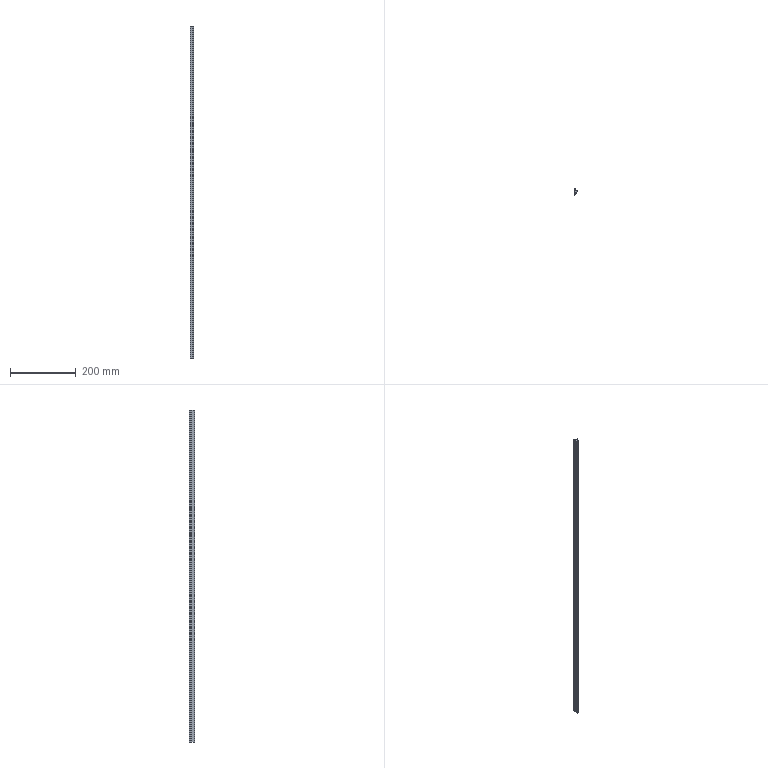Part | SolidWorks | features BaseBody 1, MoveFace 1 | 1 solid | 20 faces | box 10.8 x 17.5 x 1010 mm | volume 79589 mm3 | cylinder 11 | plane 9 | commonest cylinder face diameters 1.6 x2 14 x2 0.4 x1 0.6 x1 0.8 x1 2.6 x1
STEP:
#1=CARTESIAN_POINT('',(-3.236,-11.055,910.));
#2=VERTEX_POINT('',#1);
#3=CARTESIAN_POINT('',(-4.3,-10.3,910.));
#4=VERTEX_POINT('',#3);
#5=CARTESIAN_POINT('',(-3.5,-10.3,910.));
#6=DIRECTION('',(0.,0.,-1.));
#7=DIRECTION('',(1.,0.,0.));
#8=AXIS2_PLACEMENT_3D('',#5,#6,#7);
#9=CIRCLE('',#8,0.8);
#10=EDGE_CURVE('',#2,#4,#9,.T.);
#11=ORIENTED_EDGE('',*,*,#10,.T.);
#12=CARTESIAN_POINT('',(-4.3,-10.3,-100.));
#13=VERTEX_POINT('',#12);
#14=CARTESIAN_POINT('',(-4.3,-10.3,-100.));
#15=DIRECTION('',(0.,0.,-1.));
#16=VECTOR('',#15,1000.);
#17=LINE('',#14,#16);
#18=EDGE_CURVE('',#4,#13,#17,.T.);
#19=ORIENTED_EDGE('',*,*,#18,.T.);
#20=CARTESIAN_POINT('',(-3.236,-11.055,-100.));
#21=VERTEX_POINT('',#20);
#22=CARTESIAN_POINT('',(-3.5,-10.3,-100.));
#23=DIRECTION('',(0.,0.,1.));
#24=DIRECTION('',(-1.,0.,0.));
#25=AXIS2_PLACEMENT_3D('',#22,#23,#24);
#26=CIRCLE('',#25,0.8);
#27=EDGE_CURVE('',#13,#21,#26,.T.);
#28=ORIENTED_EDGE('',*,*,#27,.T.);
#29=CARTESIAN_POINT('',(-3.236,-11.055,-100.));
#30=DIRECTION('',(0.,0.,-1.));
#31=VECTOR('',#30,1000.);
#32=LINE('',#29,#31);
#33=EDGE_CURVE('',#2,#21,#32,.T.);
#34=ORIENTED_EDGE('',*,*,#33,.F.);
#35=EDGE_LOOP('',(#11,#19,#28,#34));
#36=FACE_OUTER_BOUND('',#35,.T.);
#37=CARTESIAN_POINT('',(-3.5,-10.3,-100.));
#38=DIRECTION('',(0.,0.,-1.));
#39=DIRECTION('',(-1.,0.,0.));
#40=AXIS2_PLACEMENT_3D('',#37,#38,#39);
#41=CYLINDRICAL_SURFACE('',#40,0.8);
#42=ADVANCED_FACE('',(#36),#41,.T.);
#43=CARTESIAN_POINT('',(1.184,-6.397,-100.));
#44=VERTEX_POINT('',#43);
#45=CARTESIAN_POINT('',(-5.702,-4.29,-100.));
#46=DIRECTION('',(0.,0.,1.));
#47=DIRECTION('',(-1.,0.,0.));
#48=AXIS2_PLACEMENT_3D('',#45,#46,#47);
#49=CIRCLE('',#48,7.201);
#50=EDGE_CURVE('',#21,#44,#49,.T.);
#51=ORIENTED_EDGE('',*,*,#50,.T.);
#52=CARTESIAN_POINT('',(1.184,-6.397,910.));
#53=VERTEX_POINT('',#52);
#54=CARTESIAN_POINT('',(1.184,-6.397,-100.));
#55=DIRECTION('',(0.,0.,1.));
#56=VECTOR('',#55,1000.);
#57=LINE('',#54,#56);
#58=EDGE_CURVE('',#44,#53,#57,.T.);
#59=ORIENTED_EDGE('',*,*,#58,.T.);
#60=CARTESIAN_POINT('',(-5.702,-4.29,910.));
#61=DIRECTION('',(0.,0.,-1.));
#62=DIRECTION('',(1.,0.,0.));
#63=AXIS2_PLACEMENT_3D('',#60,#61,#62);
#64=CIRCLE('',#63,7.201);
#65=EDGE_CURVE('',#53,#2,#64,.T.);
#66=ORIENTED_EDGE('',*,*,#65,.T.);
#67=ORIENTED_EDGE('',*,*,#33,.T.);
#68=EDGE_LOOP('',(#51,#59,#66,#67));
#69=FACE_OUTER_BOUND('',#68,.T.);
#70=CARTESIAN_POINT('',(-5.702,-4.29,-100.));
#71=DIRECTION('',(0.,0.,-1.));
#72=DIRECTION('',(-1.,0.,0.));
#73=AXIS2_PLACEMENT_3D('',#70,#71,#72);
#74=CYLINDRICAL_SURFACE('',#73,7.201);
#75=ADVANCED_FACE('',(#69),#74,.T.);
#76=CARTESIAN_POINT('',(0.9,-6.,-100.));
#77=VERTEX_POINT('',#76);
#78=CARTESIAN_POINT('',(0.9,-6.3,-100.));
#79=DIRECTION('',(0.,0.,1.));
#80=DIRECTION('',(-1.,0.,0.));
#81=AXIS2_PLACEMENT_3D('',#78,#79,#80);
#82=CIRCLE('',#81,0.3);
#83=EDGE_CURVE('',#44,#77,#82,.T.);
#84=ORIENTED_EDGE('',*,*,#83,.T.);
#85=CARTESIAN_POINT('',(0.9,-6.,910.));
#86=VERTEX_POINT('',#85);
#87=CARTESIAN_POINT('',(0.9,-6.,-100.));
#88=DIRECTION('',(0.,0.,1.));
#89=VECTOR('',#88,1000.);
#90=LINE('',#87,#89);
#91=EDGE_CURVE('',#77,#86,#90,.T.);
#92=ORIENTED_EDGE('',*,*,#91,.T.);
#93=CARTESIAN_POINT('',(0.9,-6.3,910.));
#94=DIRECTION('',(0.,0.,-1.));
#95=DIRECTION('',(1.,0.,0.));
#96=AXIS2_PLACEMENT_3D('',#93,#94,#95);
#97=CIRCLE('',#96,0.3);
#98=EDGE_CURVE('',#86,#53,#97,.T.);
#99=ORIENTED_EDGE('',*,*,#98,.T.);
#100=ORIENTED_EDGE('',*,*,#58,.F.);
#101=EDGE_LOOP('',(#84,#92,#99,#100));
#102=FACE_OUTER_BOUND('',#101,.T.);
#103=CARTESIAN_POINT('',(0.9,-6.3,-100.));
#104=DIRECTION('',(0.,0.,-1.));
#105=DIRECTION('',(-1.,0.,0.));
#106=AXIS2_PLACEMENT_3D('',#103,#104,#105);
#107=CYLINDRICAL_SURFACE('',#106,0.3);
#108=ADVANCED_FACE('',(#102),#107,.T.);
#109=CARTESIAN_POINT('',(-2.5,-0.5,-100.));
#110=VERTEX_POINT('',#109);
#111=CARTESIAN_POINT('',(-2.5,-6.153,-100.));
#112=VERTEX_POINT('',#111);
#113=CARTESIAN_POINT('',(-2.5,-6.397,-100.));
#114=DIRECTION('',(0.,-1.,0.));
#115=VECTOR('',#114,1000.);
#116=LINE('',#113,#115);
#117=EDGE_CURVE('',#110,#112,#116,.T.);
#118=ORIENTED_EDGE('',*,*,#117,.F.);
#119=CARTESIAN_POINT('',(-4.2,1.695,-100.));
#120=VERTEX_POINT('',#119);
#121=CARTESIAN_POINT('',(-1.701,1.875,-100.));
#122=DIRECTION('',(0.,0.,1.));
#123=DIRECTION('',(-1.,0.,0.));
#124=AXIS2_PLACEMENT_3D('',#121,#122,#123);
#125=CIRCLE('',#124,2.506);
#126=EDGE_CURVE('',#120,#110,#125,.T.);
#127=ORIENTED_EDGE('',*,*,#126,.F.);
#128=CARTESIAN_POINT('',(-4.2,5.1,-100.));
#129=VERTEX_POINT('',#128);
#130=CARTESIAN_POINT('',(-4.2,-6.397,-100.));
#131=DIRECTION('',(0.,-1.,0.));
#132=VECTOR('',#131,1000.);
#133=LINE('',#130,#132);
#134=EDGE_CURVE('',#129,#120,#133,.T.);
#135=ORIENTED_EDGE('',*,*,#134,.F.);
#136=CARTESIAN_POINT('',(-2.892,6.4,-100.));
#137=VERTEX_POINT('',#136);
#138=CARTESIAN_POINT('',(-2.9,5.1,-100.));
#139=DIRECTION('',(0.,0.,1.));
#140=DIRECTION('',(-1.,0.,0.));
#141=AXIS2_PLACEMENT_3D('',#138,#139,#140);
#142=CIRCLE('',#141,1.3);
#143=EDGE_CURVE('',#137,#129,#142,.T.);
#144=ORIENTED_EDGE('',*,*,#143,.F.);
#145=CARTESIAN_POINT('',(0.5,5.5,-100.));
#146=VERTEX_POINT('',#145);
#147=CARTESIAN_POINT('',(-2.934,-0.5999,-100.));
#148=DIRECTION('',(0.,0.,1.));
#149=DIRECTION('',(-1.,0.,0.));
#150=AXIS2_PLACEMENT_3D('',#147,#148,#149);
#151=CIRCLE('',#150,7.);
#152=EDGE_CURVE('',#146,#137,#151,.T.);
#153=ORIENTED_EDGE('',*,*,#152,.F.);
#154=CARTESIAN_POINT('',(5.5,1.7,-100.));
#155=VERTEX_POINT('',#154);
#156=CARTESIAN_POINT('',(5.5,1.7,-100.));
#157=DIRECTION('',(-0.7962,0.6051,0.));
#158=VECTOR('',#157,1000.);
#159=LINE('',#156,#158);
#160=EDGE_CURVE('',#155,#146,#159,.T.);
#161=ORIENTED_EDGE('',*,*,#160,.F.);
#162=CARTESIAN_POINT('',(6.458,-0.2215,-100.));
#163=VERTEX_POINT('',#162);
#164=CARTESIAN_POINT('',(6.458,-0.2215,-100.));
#165=DIRECTION('',(-0.4462,0.8949,0.));
#166=VECTOR('',#165,1000.);
#167=LINE('',#164,#166);
#168=EDGE_CURVE('',#163,#155,#167,.T.);
#169=ORIENTED_EDGE('',*,*,#168,.F.);
#170=CARTESIAN_POINT('',(5.895,-0.7433,-100.));
#171=VERTEX_POINT('',#170);
#172=CARTESIAN_POINT('',(6.1,-0.4,-100.));
#173=DIRECTION('',(0.,0.,1.));
#174=DIRECTION('',(-1.,0.,0.));
#175=AXIS2_PLACEMENT_3D('',#172,#173,#174);
#176=CIRCLE('',#175,0.4);
#177=EDGE_CURVE('',#171,#163,#176,.T.);
#178=ORIENTED_EDGE('',*,*,#177,.F.);
#179=CARTESIAN_POINT('',(3.,0.,-100.));
#180=VERTEX_POINT('',#179);
#181=CARTESIAN_POINT('',(2.746,-6.995,-100.));
#182=DIRECTION('',(0.,0.,-1.));
#183=DIRECTION('',(-1.,0.,0.));
#184=AXIS2_PLACEMENT_3D('',#181,#182,#183);
#185=CIRCLE('',#184,7.);
#186=EDGE_CURVE('',#180,#171,#185,.T.);
#187=ORIENTED_EDGE('',*,*,#186,.F.);
#188=CARTESIAN_POINT('',(0.,0.,-100.));
#189=VERTEX_POINT('',#188);
#190=CARTESIAN_POINT('',(-6.814,0.,-100.));
#191=DIRECTION('',(1.,0.,0.));
#192=VECTOR('',#191,1000.);
#193=LINE('',#190,#192);
#194=EDGE_CURVE('',#189,#180,#193,.T.);
#195=ORIENTED_EDGE('',*,*,#194,.F.);
#196=CARTESIAN_POINT('',(0.,-5.8,-100.));
#197=VERTEX_POINT('',#196);
#198=CARTESIAN_POINT('',(0.,-6.397,-100.));
#199=DIRECTION('',(0.,1.,0.));
#200=VECTOR('',#199,1000.);
#201=LINE('',#198,#200);
#202=EDGE_CURVE('',#197,#189,#201,.T.);
#203=ORIENTED_EDGE('',*,*,#202,.F.);
#204=CARTESIAN_POINT('',(0.2,-6.,-100.));
#205=VERTEX_POINT('',#204);
#206=CARTESIAN_POINT('',(0.2,-5.8,-100.));
#207=DIRECTION('',(0.,0.,1.));
#208=DIRECTION('',(-1.,0.,0.));
#209=AXIS2_PLACEMENT_3D('',#206,#207,#208);
#210=CIRCLE('',#209,0.2);
#211=EDGE_CURVE('',#197,#205,#210,.T.);
#212=ORIENTED_EDGE('',*,*,#211,.T.);
#213=CARTESIAN_POINT('',(-6.814,-6.,-100.));
#214=DIRECTION('',(-1.,0.,0.));
#215=VECTOR('',#214,1000.);
#216=LINE('',#213,#215);
#217=EDGE_CURVE('',#77,#205,#216,.T.);
#218=ORIENTED_EDGE('',*,*,#217,.F.);
#219=ORIENTED_EDGE('',*,*,#83,.F.);
#220=ORIENTED_EDGE('',*,*,#50,.F.);
#221=ORIENTED_EDGE('',*,*,#27,.F.);
#222=CARTESIAN_POINT('',(-3.998,-9.674,-100.));
#223=VERTEX_POINT('',#222);
#224=CARTESIAN_POINT('',(-3.5,-10.3,-100.));
#225=DIRECTION('',(0.,0.,1.));
#226=DIRECTION('',(-1.,0.,0.));
#227=AXIS2_PLACEMENT_3D('',#224,#225,#226);
#228=CIRCLE('',#227,0.8);
#229=EDGE_CURVE('',#223,#13,#228,.T.);
#230=ORIENTED_EDGE('',*,*,#229,.F.);
#231=CARTESIAN_POINT('',(-6.814,-6.397,-100.));
#232=DIRECTION('',(0.,0.,-1.));
#233=DIRECTION('',(-1.,0.,0.));
#234=AXIS2_PLACEMENT_3D('',#231,#232,#233);
#235=CIRCLE('',#234,4.321);
#236=EDGE_CURVE('',#112,#223,#235,.T.);
#237=ORIENTED_EDGE('',*,*,#236,.F.);
#238=EDGE_LOOP('',(#118,#127,#135,#144,#153,#161,#169,#178,#187,#195,#203,#212,#218,#219,#220,#221,#230,#237));
#239=FACE_OUTER_BOUND('',#238,.T.);
#240=CARTESIAN_POINT('',(-6.814,-6.397,-100.));
#241=DIRECTION('',(0.,0.,1.));
#242=DIRECTION('',(1.,0.,0.));
#243=AXIS2_PLACEMENT_3D('',#240,#241,#242);
#244=PLANE('',#243);
#245=ADVANCED_FACE('',(#239),#244,.F.);
#246=ORIENTED_EDGE('',*,*,#18,.F.);
#247=CARTESIAN_POINT('',(-3.998,-9.674,910.));
#248=VERTEX_POINT('',#247);
#249=CARTESIAN_POINT('',(-3.5,-10.3,910.));
#250=DIRECTION('',(0.,0.,-1.));
#251=DIRECTION('',(1.,0.,0.));
#252=AXIS2_PLACEMENT_3D('',#249,#250,#251);
#253=CIRCLE('',#252,0.8);
#254=EDGE_CURVE('',#4,#248,#253,.T.);
#255=ORIENTED_EDGE('',*,*,#254,.T.);
#256=CARTESIAN_POINT('',(-3.998,-9.674,-100.));
#257=DIRECTION('',(0.,0.,-1.));
#258=VECTOR('',#257,1000.);
#259=LINE('',#256,#258);
#260=EDGE_CURVE('',#248,#223,#259,.T.);
#261=ORIENTED_EDGE('',*,*,#260,.T.);
#262=ORIENTED_EDGE('',*,*,#229,.T.);
#263=EDGE_LOOP('',(#246,#255,#261,#262));
#264=FACE_OUTER_BOUND('',#263,.T.);
#265=CARTESIAN_POINT('',(-3.5,-10.3,-100.));
#266=DIRECTION('',(0.,0.,-1.));
#267=DIRECTION('',(-1.,0.,0.));
#268=AXIS2_PLACEMENT_3D('',#265,#266,#267);
#269=CYLINDRICAL_SURFACE('',#268,0.8);
#270=ADVANCED_FACE('',(#264),#269,.T.);
#271=CARTESIAN_POINT('',(-4.2,1.695,910.));
#272=VERTEX_POINT('',#271);
#273=CARTESIAN_POINT('',(-2.5,-0.5,910.));
#274=VERTEX_POINT('',#273);
#275=CARTESIAN_POINT('',(-1.701,1.875,910.));
#276=DIRECTION('',(0.,0.,1.));
#277=DIRECTION('',(1.,0.,0.));
#278=AXIS2_PLACEMENT_3D('',#275,#276,#277);
#279=CIRCLE('',#278,2.506);
#280=EDGE_CURVE('',#272,#274,#279,.T.);
#281=ORIENTED_EDGE('',*,*,#280,.T.);
#282=CARTESIAN_POINT('',(-2.5,-6.153,910.));
#283=VERTEX_POINT('',#282);
#284=CARTESIAN_POINT('',(-2.5,-6.397,910.));
#285=DIRECTION('',(0.,-1.,0.));
#286=VECTOR('',#285,1000.);
#287=LINE('',#284,#286);
#288=EDGE_CURVE('',#274,#283,#287,.T.);
#289=ORIENTED_EDGE('',*,*,#288,.T.);
#290=CARTESIAN_POINT('',(-6.814,-6.397,910.));
#291=DIRECTION('',(0.,0.,-1.));
#292=DIRECTION('',(1.,0.,0.));
#293=AXIS2_PLACEMENT_3D('',#290,#291,#292);
#294=CIRCLE('',#293,4.321);
#295=EDGE_CURVE('',#283,#248,#294,.T.);
#296=ORIENTED_EDGE('',*,*,#295,.T.);
#297=ORIENTED_EDGE('',*,*,#254,.F.);
#298=ORIENTED_EDGE('',*,*,#10,.F.);
#299=ORIENTED_EDGE('',*,*,#65,.F.);
#300=ORIENTED_EDGE('',*,*,#98,.F.);
#301=CARTESIAN_POINT('',(0.2,-6.,910.));
#302=VERTEX_POINT('',#301);
#303=CARTESIAN_POINT('',(-6.814,-6.,910.));
#304=DIRECTION('',(-1.,0.,0.));
#305=VECTOR('',#304,1000.);
#306=LINE('',#303,#305);
#307=EDGE_CURVE('',#86,#302,#306,.T.);
#308=ORIENTED_EDGE('',*,*,#307,.T.);
#309=CARTESIAN_POINT('',(0.,-5.8,910.));
#310=VERTEX_POINT('',#309);
#311=CARTESIAN_POINT('',(0.2,-5.8,910.));
#312=DIRECTION('',(0.,0.,-1.));
#313=DIRECTION('',(1.,0.,0.));
#314=AXIS2_PLACEMENT_3D('',#311,#312,#313);
#315=CIRCLE('',#314,0.2);
#316=EDGE_CURVE('',#302,#310,#315,.T.);
#317=ORIENTED_EDGE('',*,*,#316,.T.);
#318=CARTESIAN_POINT('',(0.,0.,910.));
#319=VERTEX_POINT('',#318);
#320=CARTESIAN_POINT('',(0.,-6.397,910.));
#321=DIRECTION('',(0.,1.,0.));
#322=VECTOR('',#321,1000.);
#323=LINE('',#320,#322);
#324=EDGE_CURVE('',#310,#319,#323,.T.);
#325=ORIENTED_EDGE('',*,*,#324,.T.);
#326=CARTESIAN_POINT('',(3.,0.,910.));
#327=VERTEX_POINT('',#326);
#328=CARTESIAN_POINT('',(-6.814,0.,910.));
#329=DIRECTION('',(1.,0.,0.));
#330=VECTOR('',#329,1000.);
#331=LINE('',#328,#330);
#332=EDGE_CURVE('',#319,#327,#331,.T.);
#333=ORIENTED_EDGE('',*,*,#332,.T.);
#334=CARTESIAN_POINT('',(5.895,-0.7433,910.));
#335=VERTEX_POINT('',#334);
#336=CARTESIAN_POINT('',(2.746,-6.995,910.));
#337=DIRECTION('',(0.,0.,-1.));
#338=DIRECTION('',(1.,0.,0.));
#339=AXIS2_PLACEMENT_3D('',#336,#337,#338);
#340=CIRCLE('',#339,7.);
#341=EDGE_CURVE('',#327,#335,#340,.T.);
#342=ORIENTED_EDGE('',*,*,#341,.T.);
#343=CARTESIAN_POINT('',(6.458,-0.2215,910.));
#344=VERTEX_POINT('',#343);
#345=CARTESIAN_POINT('',(6.1,-0.4,910.));
#346=DIRECTION('',(0.,0.,-1.));
#347=DIRECTION('',(1.,0.,0.));
#348=AXIS2_PLACEMENT_3D('',#345,#346,#347);
#349=CIRCLE('',#348,0.4);
#350=EDGE_CURVE('',#344,#335,#349,.T.);
#351=ORIENTED_EDGE('',*,*,#350,.F.);
#352=CARTESIAN_POINT('',(5.5,1.7,910.));
#353=VERTEX_POINT('',#352);
#354=CARTESIAN_POINT('',(6.282,0.1323,910.));
#355=DIRECTION('',(-0.4462,0.8949,0.));
#356=VECTOR('',#355,1000.);
#357=LINE('',#354,#356);
#358=EDGE_CURVE('',#344,#353,#357,.T.);
#359=ORIENTED_EDGE('',*,*,#358,.T.);
#360=CARTESIAN_POINT('',(0.5,5.5,910.));
#361=VERTEX_POINT('',#360);
#362=CARTESIAN_POINT('',(1.595,4.668,910.));
#363=DIRECTION('',(-0.7962,0.6051,0.));
#364=VECTOR('',#363,1000.);
#365=LINE('',#362,#364);
#366=EDGE_CURVE('',#353,#361,#365,.T.);
#367=ORIENTED_EDGE('',*,*,#366,.T.);
#368=CARTESIAN_POINT('',(-2.892,6.4,910.));
#369=VERTEX_POINT('',#368);
#370=CARTESIAN_POINT('',(-2.934,-0.5999,910.));
#371=DIRECTION('',(0.,0.,1.));
#372=DIRECTION('',(1.,0.,0.));
#373=AXIS2_PLACEMENT_3D('',#370,#371,#372);
#374=CIRCLE('',#373,7.);
#375=EDGE_CURVE('',#361,#369,#374,.T.);
#376=ORIENTED_EDGE('',*,*,#375,.T.);
#377=CARTESIAN_POINT('',(-4.2,5.1,910.));
#378=VERTEX_POINT('',#377);
#379=CARTESIAN_POINT('',(-2.9,5.1,910.));
#380=DIRECTION('',(0.,0.,1.));
#381=DIRECTION('',(1.,0.,0.));
#382=AXIS2_PLACEMENT_3D('',#379,#380,#381);
#383=CIRCLE('',#382,1.3);
#384=EDGE_CURVE('',#369,#378,#383,.T.);
#385=ORIENTED_EDGE('',*,*,#384,.T.);
#386=CARTESIAN_POINT('',(-4.2,-6.397,910.));
#387=DIRECTION('',(0.,-1.,0.));
#388=VECTOR('',#387,1000.);
#389=LINE('',#386,#388);
#390=EDGE_CURVE('',#378,#272,#389,.T.);
#391=ORIENTED_EDGE('',*,*,#390,.T.);
#392=EDGE_LOOP('',(#281,#289,#296,#297,#298,#299,#300,#308,#317,#325,#333,#342,#351,#359,#367,#376,#385,#391));
#393=FACE_OUTER_BOUND('',#392,.T.);
#394=CARTESIAN_POINT('',(-6.814,-6.397,910.));
#395=DIRECTION('',(0.,0.,1.));
#396=DIRECTION('',(1.,0.,0.));
#397=AXIS2_PLACEMENT_3D('',#394,#395,#396);
#398=PLANE('',#397);
#399=ADVANCED_FACE('',(#393),#398,.T.);
#400=ORIENTED_EDGE('',*,*,#217,.T.);
#401=CARTESIAN_POINT('',(0.2,-6.,-100.));
#402=DIRECTION('',(0.,0.,1.));
#403=VECTOR('',#402,1000.);
#404=LINE('',#401,#403);
#405=EDGE_CURVE('',#205,#302,#404,.T.);
#406=ORIENTED_EDGE('',*,*,#405,.T.);
#407=ORIENTED_EDGE('',*,*,#307,.F.);
#408=ORIENTED_EDGE('',*,*,#91,.F.);
#409=EDGE_LOOP('',(#400,#406,#407,#408));
#410=FACE_OUTER_BOUND('',#409,.T.);
#411=CARTESIAN_POINT('',(0.9,-6.,-100.));
#412=DIRECTION('',(0.,1.,0.));
#413=DIRECTION('',(0.,0.,1.));
#414=AXIS2_PLACEMENT_3D('',#411,#412,#413);
#415=PLANE('',#414);
#416=ADVANCED_FACE('',(#410),#415,.T.);
#417=CARTESIAN_POINT('',(-2.5,-6.153,-100.));
#418=DIRECTION('',(0.,0.,1.));
#419=VECTOR('',#418,1000.);
#420=LINE('',#417,#419);
#421=EDGE_CURVE('',#112,#283,#420,.T.);
#422=ORIENTED_EDGE('',*,*,#421,.F.);
#423=ORIENTED_EDGE('',*,*,#236,.T.);
#424=ORIENTED_EDGE('',*,*,#260,.F.);
#425=ORIENTED_EDGE('',*,*,#295,.F.);
#426=EDGE_LOOP('',(#422,#423,#424,#425));
#427=FACE_OUTER_BOUND('',#426,.T.);
#428=CARTESIAN_POINT('',(-6.814,-6.397,-100.));
#429=DIRECTION('',(0.,0.,-1.));
#430=DIRECTION('',(-1.,0.,0.));
#431=AXIS2_PLACEMENT_3D('',#428,#429,#430);
#432=CYLINDRICAL_SURFACE('',#431,4.321);
#433=ADVANCED_FACE('',(#427),#432,.F.);
#434=ORIENTED_EDGE('',*,*,#117,.T.);
#435=ORIENTED_EDGE('',*,*,#421,.T.);
#436=ORIENTED_EDGE('',*,*,#288,.F.);
#437=CARTESIAN_POINT('',(-2.5,-0.5,-100.));
#438=DIRECTION('',(0.,0.,-1.));
#439=VECTOR('',#438,1000.);
#440=LINE('',#437,#439);
#441=EDGE_CURVE('',#274,#110,#440,.T.);
#442=ORIENTED_EDGE('',*,*,#441,.T.);
#443=EDGE_LOOP('',(#434,#435,#436,#442));
#444=FACE_OUTER_BOUND('',#443,.T.);
#445=CARTESIAN_POINT('',(-2.5,-0.5,-100.));
#446=DIRECTION('',(-1.,0.,0.));
#447=DIRECTION('',(0.,0.,1.));
#448=AXIS2_PLACEMENT_3D('',#445,#446,#447);
#449=PLANE('',#448);
#450=ADVANCED_FACE('',(#444),#449,.T.);
#451=ORIENTED_EDGE('',*,*,#126,.T.);
#452=ORIENTED_EDGE('',*,*,#441,.F.);
#453=ORIENTED_EDGE('',*,*,#280,.F.);
#454=CARTESIAN_POINT('',(-4.2,1.695,-100.));
#455=DIRECTION('',(0.,0.,-1.));
#456=VECTOR('',#455,1000.);
#457=LINE('',#454,#456);
#458=EDGE_CURVE('',#272,#120,#457,.T.);
#459=ORIENTED_EDGE('',*,*,#458,.T.);
#460=EDGE_LOOP('',(#451,#452,#453,#459));
#461=FACE_OUTER_BOUND('',#460,.T.);
#462=CARTESIAN_POINT('',(-1.701,1.875,-100.));
#463=DIRECTION('',(0.,0.,-1.));
#464=DIRECTION('',(-1.,0.,0.));
#465=AXIS2_PLACEMENT_3D('',#462,#463,#464);
#466=CYLINDRICAL_SURFACE('',#465,2.506);
#467=ADVANCED_FACE('',(#461),#466,.T.);
#468=ORIENTED_EDGE('',*,*,#134,.T.);
#469=ORIENTED_EDGE('',*,*,#458,.F.);
#470=ORIENTED_EDGE('',*,*,#390,.F.);
#471=CARTESIAN_POINT('',(-4.2,5.1,-100.));
#472=DIRECTION('',(0.,0.,-1.));
#473=VECTOR('',#472,1000.);
#474=LINE('',#471,#473);
#475=EDGE_CURVE('',#378,#129,#474,.T.);
#476=ORIENTED_EDGE('',*,*,#475,.T.);
#477=EDGE_LOOP('',(#468,#469,#470,#476));
#478=FACE_OUTER_BOUND('',#477,.T.);
#479=CARTESIAN_POINT('',(-4.2,5.1,-100.));
#480=DIRECTION('',(-1.,0.,0.));
#481=DIRECTION('',(0.,0.,1.));
#482=AXIS2_PLACEMENT_3D('',#479,#480,#481);
#483=PLANE('',#482);
#484=ADVANCED_FACE('',(#478),#483,.T.);
#485=ORIENTED_EDGE('',*,*,#143,.T.);
#486=ORIENTED_EDGE('',*,*,#475,.F.);
#487=ORIENTED_EDGE('',*,*,#384,.F.);
#488=CARTESIAN_POINT('',(-2.892,6.4,-100.));
#489=DIRECTION('',(0.,0.,-1.));
#490=VECTOR('',#489,1000.);
#491=LINE('',#488,#490);
#492=EDGE_CURVE('',#369,#137,#491,.T.);
#493=ORIENTED_EDGE('',*,*,#492,.T.);
#494=EDGE_LOOP('',(#485,#486,#487,#493));
#495=FACE_OUTER_BOUND('',#494,.T.);
#496=CARTESIAN_POINT('',(-2.9,5.1,-100.));
#497=DIRECTION('',(0.,0.,-1.));
#498=DIRECTION('',(-1.,0.,0.));
#499=AXIS2_PLACEMENT_3D('',#496,#497,#498);
#500=CYLINDRICAL_SURFACE('',#499,1.3);
#501=ADVANCED_FACE('',(#495),#500,.T.);
#502=ORIENTED_EDGE('',*,*,#152,.T.);
#503=ORIENTED_EDGE('',*,*,#492,.F.);
#504=ORIENTED_EDGE('',*,*,#375,.F.);
#505=CARTESIAN_POINT('',(0.5,5.5,-100.));
#506=DIRECTION('',(0.,0.,-1.));
#507=VECTOR('',#506,1000.);
#508=LINE('',#505,#507);
#509=EDGE_CURVE('',#361,#146,#508,.T.);
#510=ORIENTED_EDGE('',*,*,#509,.T.);
#511=EDGE_LOOP('',(#502,#503,#504,#510));
#512=FACE_OUTER_BOUND('',#511,.T.);
#513=CARTESIAN_POINT('',(-2.934,-0.5999,-100.));
#514=DIRECTION('',(0.,0.,-1.));
#515=DIRECTION('',(-1.,0.,0.));
#516=AXIS2_PLACEMENT_3D('',#513,#514,#515);
#517=CYLINDRICAL_SURFACE('',#516,7.);
#518=ADVANCED_FACE('',(#512),#517,.T.);
#519=ORIENTED_EDGE('',*,*,#160,.T.);
#520=ORIENTED_EDGE('',*,*,#509,.F.);
#521=ORIENTED_EDGE('',*,*,#366,.F.);
#522=CARTESIAN_POINT('',(5.5,1.7,-100.));
#523=DIRECTION('',(0.,0.,-1.));
#524=VECTOR('',#523,1000.);
#525=LINE('',#522,#524);
#526=EDGE_CURVE('',#353,#155,#525,.T.);
#527=ORIENTED_EDGE('',*,*,#526,.T.);
#528=EDGE_LOOP('',(#519,#520,#521,#527));
#529=FACE_OUTER_BOUND('',#528,.T.);
#530=CARTESIAN_POINT('',(5.5,1.7,-100.));
#531=DIRECTION('',(0.6051,0.7962,0.));
#532=DIRECTION('',(-0.7962,0.6051,0.));
#533=AXIS2_PLACEMENT_3D('',#530,#531,#532);
#534=PLANE('',#533);
#535=ADVANCED_FACE('',(#529),#534,.T.);
#536=ORIENTED_EDGE('',*,*,#168,.T.);
#537=ORIENTED_EDGE('',*,*,#526,.F.);
#538=ORIENTED_EDGE('',*,*,#358,.F.);
#539=CARTESIAN_POINT('',(6.458,-0.2215,-100.));
#540=DIRECTION('',(0.,0.,-1.));
#541=VECTOR('',#540,1000.);
#542=LINE('',#539,#541);
#543=EDGE_CURVE('',#344,#163,#542,.T.);
#544=ORIENTED_EDGE('',*,*,#543,.T.);
#545=EDGE_LOOP('',(#536,#537,#538,#544));
#546=FACE_OUTER_BOUND('',#545,.T.);
#547=CARTESIAN_POINT('',(6.458,-0.2215,-100.));
#548=DIRECTION('',(0.8949,0.4462,0.));
#549=DIRECTION('',(-0.4462,0.8949,0.));
#550=AXIS2_PLACEMENT_3D('',#547,#548,#549);
#551=PLANE('',#550);
#552=ADVANCED_FACE('',(#546),#551,.T.);
#553=CARTESIAN_POINT('',(3.,0.,-100.));
#554=DIRECTION('',(0.,0.,1.));
#555=VECTOR('',#554,1000.);
#556=LINE('',#553,#555);
#557=EDGE_CURVE('',#180,#327,#556,.T.);
#558=ORIENTED_EDGE('',*,*,#557,.F.);
#559=ORIENTED_EDGE('',*,*,#186,.T.);
#560=CARTESIAN_POINT('',(5.895,-0.7433,-100.));
#561=DIRECTION('',(0.,0.,-1.));
#562=VECTOR('',#561,1000.);
#563=LINE('',#560,#562);
#564=EDGE_CURVE('',#335,#171,#563,.T.);
#565=ORIENTED_EDGE('',*,*,#564,.F.);
#566=ORIENTED_EDGE('',*,*,#341,.F.);
#567=EDGE_LOOP('',(#558,#559,#565,#566));
#568=FACE_OUTER_BOUND('',#567,.T.);
#569=CARTESIAN_POINT('',(2.746,-6.995,-100.));
#570=DIRECTION('',(0.,0.,-1.));
#571=DIRECTION('',(-1.,0.,0.));
#572=AXIS2_PLACEMENT_3D('',#569,#570,#571);
#573=CYLINDRICAL_SURFACE('',#572,7.);
#574=ADVANCED_FACE('',(#568),#573,.F.);
#575=ORIENTED_EDGE('',*,*,#194,.T.);
#576=ORIENTED_EDGE('',*,*,#557,.T.);
#577=ORIENTED_EDGE('',*,*,#332,.F.);
#578=CARTESIAN_POINT('',(0.,0.,-100.));
#579=DIRECTION('',(0.,0.,-1.));
#580=VECTOR('',#579,1000.);
#581=LINE('',#578,#580);
#582=EDGE_CURVE('',#319,#189,#581,.T.);
#583=ORIENTED_EDGE('',*,*,#582,.T.);
#584=EDGE_LOOP('',(#575,#576,#577,#583));
#585=FACE_OUTER_BOUND('',#584,.T.);
#586=CARTESIAN_POINT('',(0.,0.,-100.));
#587=DIRECTION('',(0.,-1.,0.));
#588=DIRECTION('',(0.,0.,-1.));
#589=AXIS2_PLACEMENT_3D('',#586,#587,#588);
#590=PLANE('',#589);
#591=ADVANCED_FACE('',(#585),#590,.T.);
#592=ORIENTED_EDGE('',*,*,#202,.T.);
#593=ORIENTED_EDGE('',*,*,#582,.F.);
#594=ORIENTED_EDGE('',*,*,#324,.F.);
#595=CARTESIAN_POINT('',(0.,-5.8,-100.));
#596=DIRECTION('',(0.,0.,-1.));
#597=VECTOR('',#596,1000.);
#598=LINE('',#595,#597);
#599=EDGE_CURVE('',#310,#197,#598,.T.);
#600=ORIENTED_EDGE('',*,*,#599,.T.);
#601=EDGE_LOOP('',(#592,#593,#594,#600));
#602=FACE_OUTER_BOUND('',#601,.T.);
#603=CARTESIAN_POINT('',(0.,-5.8,-100.));
#604=DIRECTION('',(1.,0.,0.));
#605=DIRECTION('',(0.,0.,-1.));
#606=AXIS2_PLACEMENT_3D('',#603,#604,#605);
#607=PLANE('',#606);
#608=ADVANCED_FACE('',(#602),#607,.T.);
#609=ORIENTED_EDGE('',*,*,#405,.F.);
#610=ORIENTED_EDGE('',*,*,#211,.F.);
#611=ORIENTED_EDGE('',*,*,#599,.F.);
#612=ORIENTED_EDGE('',*,*,#316,.F.);
#613=EDGE_LOOP('',(#609,#610,#611,#612));
#614=FACE_OUTER_BOUND('',#613,.T.);
#615=CARTESIAN_POINT('',(0.2,-5.8,-100.));
#616=DIRECTION('',(0.,0.,-1.));
#617=DIRECTION('',(-1.,0.,0.));
#618=AXIS2_PLACEMENT_3D('',#615,#616,#617);
#619=CYLINDRICAL_SURFACE('',#618,0.2);
#620=ADVANCED_FACE('',(#614),#619,.F.);
#621=ORIENTED_EDGE('',*,*,#177,.T.);
#622=ORIENTED_EDGE('',*,*,#543,.F.);
#623=ORIENTED_EDGE('',*,*,#350,.T.);
#624=ORIENTED_EDGE('',*,*,#564,.T.);
#625=EDGE_LOOP('',(#621,#622,#623,#624));
#626=FACE_OUTER_BOUND('',#625,.T.);
#627=CARTESIAN_POINT('',(6.1,-0.4,-100.));
#628=DIRECTION('',(0.,0.,-1.));
#629=DIRECTION('',(-1.,0.,0.));
#630=AXIS2_PLACEMENT_3D('',#627,#628,#629);
#631=CYLINDRICAL_SURFACE('',#630,0.4);
#632=ADVANCED_FACE('',(#626),#631,.T.);
#633=CLOSED_SHELL('',(#42,#75,#108,#245,#270,#399,#416,#433,#450,#467,#484,#501,#518,#535,#552,#574,#591,#608,#620,#632));
#634=MANIFOLD_SOLID_BREP('',#633);
#635=CARTESIAN_POINT('',(0.,0.,0.));
#636=DIRECTION('',(0.,0.,1.));
#637=DIRECTION('',(1.,0.,0.));
#638=AXIS2_PLACEMENT_3D('',#635,#636,#637);
#639=(LENGTH_UNIT()NAMED_UNIT(*)SI_UNIT(.MILLI.,.METRE.));
#640=UNCERTAINTY_MEASURE_WITH_UNIT(LENGTH_MEASURE(0.00001),#639,'','');
#641=(NAMED_UNIT(*)PLANE_ANGLE_UNIT()SI_UNIT($,.RADIAN.));
#642=(NAMED_UNIT(*)SI_UNIT($,.STERADIAN.)SOLID_ANGLE_UNIT());
#643=(GEOMETRIC_REPRESENTATION_CONTEXT(3)GLOBAL_UNCERTAINTY_ASSIGNED_CONTEXT((#640))GLOBAL_UNIT_ASSIGNED_CONTEXT((#639,#641,#642))REPRESENTATION_CONTEXT('',''));
#644=ADVANCED_BREP_SHAPE_REPRESENTATION('',(#634,#638),#643);